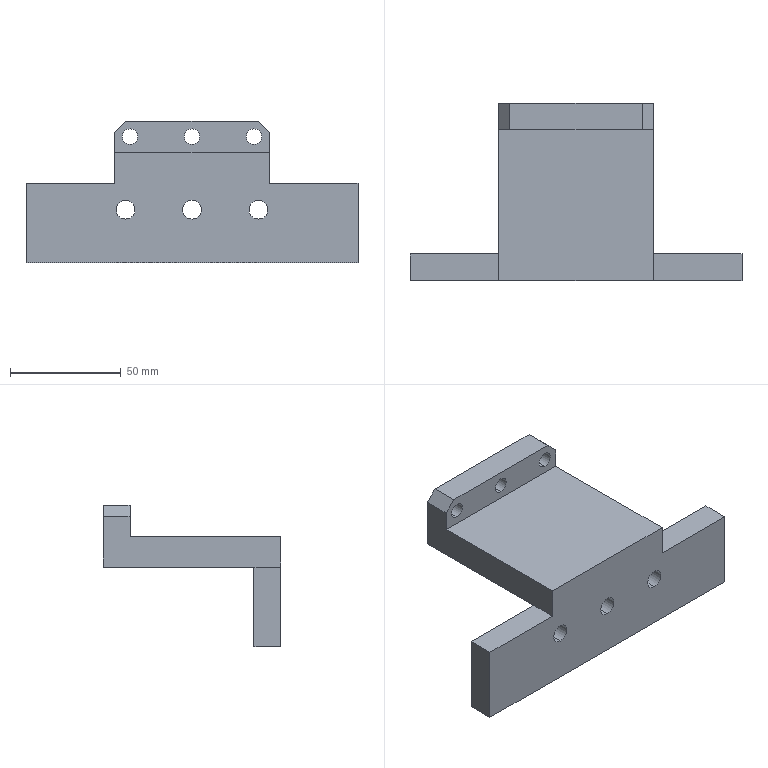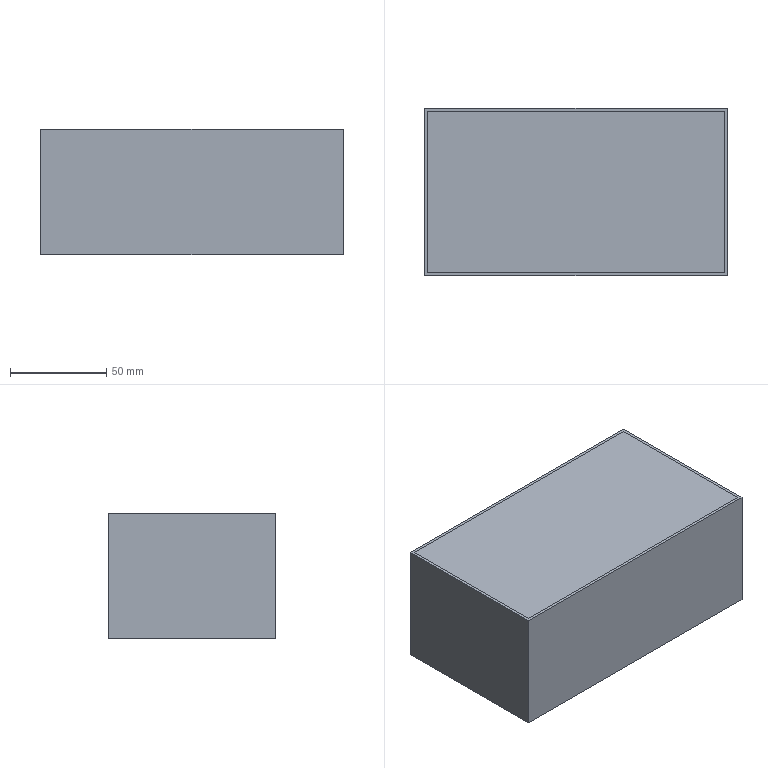CAM job | NX | 3+2 milling, drilling | part box 150 x 80 x 64 mm | stock box 157 x 87 x 65 mm
Tools:
number,name,description,diameter,corner_radius,flute_length,length,flutes
1,D63,Milling Tool-5 Parameters,63.0,0.0,50.0,75.0,2
9,D12,Milling Tool-5 Parameters,12.0,0.0,50.0,75.0,2
10,D10,Milling Tool-5 Parameters,10.0,0.0,50.0,75.0,2
5,D4R0.5,Milling Tool-5 Parameters,4.0,0.5,50.0,75.0,2
7,D6A45,Milling Tool-5 Parameters,6.0,0.0,50.0,75.0,2
Operations:
program,operation,operation_type,tool,method,geometry_group,spindle_rpm,surface_speed,feed_per_tooth,feed_cut,feed_plunge,cut_length_mm,path_length_mm,cut_time_min,machine_time_min
1,FLOOR_WALL,VolumeBased25DMillingOperation,D63,METHOD,A,6500.0,1286.0,0.0962,1250.0,100.0,733.797,787.797,0.587,0.5924
1,CAVITY_MILL,CavityMilling,D12,METHOD,A,9500.0,358.0,0.1316,2500.0,1000.0,246761.61,252274.149,99.438,99.99
1,FLOOR_WALL_1,VolumeBased25DMillingOperation,D10,METHOD,A,9500.0,298.0,0.0658,1250.0,100.0,1910.122,2744.062,1.528,1.611
1,ZLEVEL_PROFILE,ZLevelMilling,D10,METHOD,A,9500.0,298.0,0.0658,1250.0,100.0,393.659,1060.264,0.3149,0.3816
1,ZLEVEL_PROFILE_COPY,ZLevelMilling,D10,METHOD,A,9500.0,298.0,0.0658,1250.0,100.0,1981.85,2539.428,1.585,1.641
1,ZLEVEL_PROFILE_1,ZLevelMilling,D4R0.5,METHOD,A,9500.0,119.0,0.1316,2500.0,1000.0,2020.294,2215.702,0.8111,0.8307
1,PLANAR_MILL,PlanarMilling,D6A45,METHOD,A,9500.0,179.0,0.0658,1250.0,100.0,181.483,237.483,0.1452,0.1508
1,PLANAR_MILL_COPY,PlanarMilling,D6A45,METHOD,A,9500.0,179.0,0.0658,1250.0,100.0,214.992,298.992,0.172,0.1804
1,PLANAR_MILL_COPY_COPY,PlanarMilling,D6A45,METHOD,A,9500.0,179.0,0.0658,1250.0,100.0,203.219,507.619,0.1626,0.193
2,FLOOR_WALL_COPY,VolumeBased25DMillingOperation,D63,METHOD,B,6500.0,1286.0,0.0962,1250.0,100.0,721.797,775.797,0.5774,0.5828
2,FLOOR_WALL_2,VolumeBased25DMillingOperation,D10,METHOD,B,9500.0,298.0,0.1316,2500.0,1000.0,78555.535,87487.334,31.582,32.475
2,FLOOR_WALL_1_COPY,VolumeBased25DMillingOperation,D10,METHOD,B,9500.0,298.0,0.0658,1250.0,100.0,1361.941,1702.942,1.09,1.124
2,FLOOR_WALL_1_COPY_COPY,VolumeBased25DMillingOperation,D10,METHOD,B,9500.0,298.0,0.0658,1250.0,100.0,262.211,742.985,0.2098,0.2578
2,PLANAR_MILL_COPY_COPY_1,PlanarMilling,D6A45,METHOD,B,9500.0,179.0,0.0658,1250.0,100.0,341.483,397.483,0.2732,0.2788
2,PLANAR_MILL_COPY_COPY_1_COPY,PlanarMilling,D6A45,METHOD,B,9500.0,179.0,0.0658,1250.0,100.0,216.227,344.227,0.173,0.1858
3,DRILLING,Operation,D6A45,METHOD,C,5000.0,94.0,0.025,250.0,0.0,24.0,385.94,0.096,0.1322